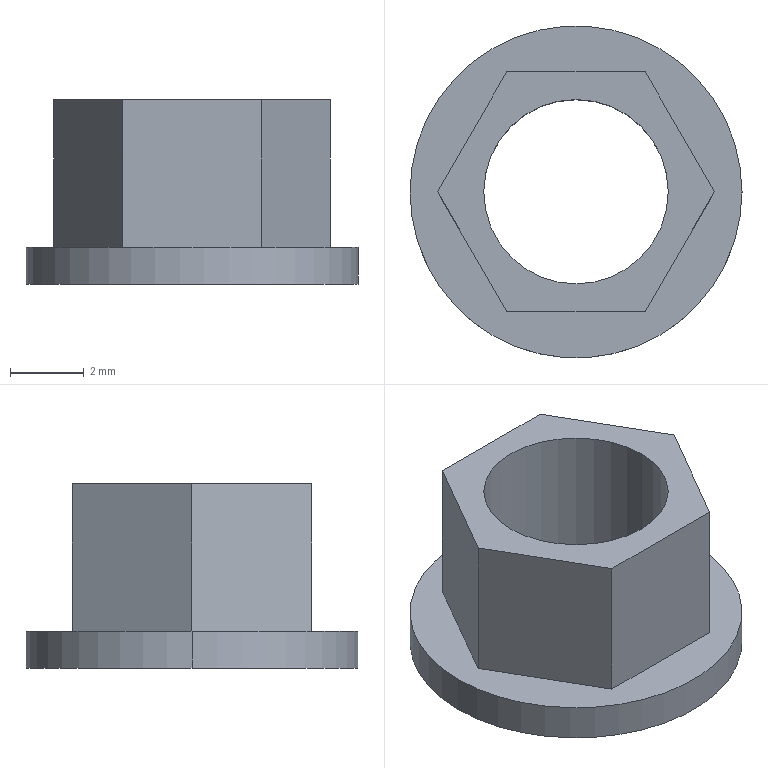Part | SolidWorks | features BaseBody 1 | 1 solid | 13 faces | box 9 x 9 x 5 mm | volume 111.801 mm3 | plane 9 | cylinder 4 | commonest cylinder face diameters 5 x2 9 x2
STEP:
#1=CARTESIAN_POINT('',(2.5,0.,0.));
#2=VERTEX_POINT('',#1);
#3=CARTESIAN_POINT('',(-2.5,0.,0.));
#4=VERTEX_POINT('',#3);
#5=CARTESIAN_POINT('',(0.,0.,0.));
#6=DIRECTION('',(0.,0.,1.));
#7=DIRECTION('',(-1.,0.,0.));
#8=AXIS2_PLACEMENT_3D('',#5,#6,#7);
#9=CIRCLE('',#8,2.5);
#10=EDGE_CURVE('',#2,#4,#9,.T.);
#11=ORIENTED_EDGE('',*,*,#10,.F.);
#12=CARTESIAN_POINT('',(2.5,0.,5.));
#13=VERTEX_POINT('',#12);
#14=CARTESIAN_POINT('',(2.5,0.,5.));
#15=DIRECTION('',(0.,0.,1.));
#16=VECTOR('',#15,1000.);
#17=LINE('',#14,#16);
#18=EDGE_CURVE('',#2,#13,#17,.T.);
#19=ORIENTED_EDGE('',*,*,#18,.T.);
#20=CARTESIAN_POINT('',(-2.5,0.,5.));
#21=VERTEX_POINT('',#20);
#22=CARTESIAN_POINT('',(0.,0.,5.));
#23=DIRECTION('',(0.,0.,-1.));
#24=DIRECTION('',(-1.,0.,0.));
#25=AXIS2_PLACEMENT_3D('',#22,#23,#24);
#26=CIRCLE('',#25,2.5);
#27=EDGE_CURVE('',#21,#13,#26,.T.);
#28=ORIENTED_EDGE('',*,*,#27,.F.);
#29=CARTESIAN_POINT('',(-2.5,0.,5.));
#30=DIRECTION('',(0.,0.,1.));
#31=VECTOR('',#30,1000.);
#32=LINE('',#29,#31);
#33=EDGE_CURVE('',#4,#21,#32,.T.);
#34=ORIENTED_EDGE('',*,*,#33,.F.);
#35=EDGE_LOOP('',(#11,#19,#28,#34));
#36=FACE_OUTER_BOUND('',#35,.T.);
#37=CARTESIAN_POINT('',(0.,0.,5.));
#38=DIRECTION('',(0.,0.,1.));
#39=DIRECTION('',(-1.,0.,0.));
#40=AXIS2_PLACEMENT_3D('',#37,#38,#39);
#41=CYLINDRICAL_SURFACE('',#40,2.5);
#42=ADVANCED_FACE('',(#36),#41,.F.);
#43=CARTESIAN_POINT('',(4.5,0.,1.));
#44=VERTEX_POINT('',#43);
#45=CARTESIAN_POINT('',(-4.5,0.,1.));
#46=VERTEX_POINT('',#45);
#47=CARTESIAN_POINT('',(0.,0.,1.));
#48=DIRECTION('',(0.,0.,1.));
#49=DIRECTION('',(-1.,0.,0.));
#50=AXIS2_PLACEMENT_3D('',#47,#48,#49);
#51=CIRCLE('',#50,4.5);
#52=EDGE_CURVE('',#44,#46,#51,.T.);
#53=ORIENTED_EDGE('',*,*,#52,.F.);
#54=CARTESIAN_POINT('',(4.5,0.,0.));
#55=VERTEX_POINT('',#54);
#56=CARTESIAN_POINT('',(4.5,0.,0.));
#57=DIRECTION('',(0.,0.,-1.));
#58=VECTOR('',#57,1000.);
#59=LINE('',#56,#58);
#60=EDGE_CURVE('',#44,#55,#59,.T.);
#61=ORIENTED_EDGE('',*,*,#60,.T.);
#62=CARTESIAN_POINT('',(-4.5,0.,0.));
#63=VERTEX_POINT('',#62);
#64=CARTESIAN_POINT('',(0.,0.,0.));
#65=DIRECTION('',(0.,0.,-1.));
#66=DIRECTION('',(-1.,0.,0.));
#67=AXIS2_PLACEMENT_3D('',#64,#65,#66);
#68=CIRCLE('',#67,4.5);
#69=EDGE_CURVE('',#63,#55,#68,.T.);
#70=ORIENTED_EDGE('',*,*,#69,.F.);
#71=CARTESIAN_POINT('',(-4.5,0.,0.));
#72=DIRECTION('',(0.,0.,-1.));
#73=VECTOR('',#72,1000.);
#74=LINE('',#71,#73);
#75=EDGE_CURVE('',#46,#63,#74,.T.);
#76=ORIENTED_EDGE('',*,*,#75,.F.);
#77=EDGE_LOOP('',(#53,#61,#70,#76));
#78=FACE_OUTER_BOUND('',#77,.T.);
#79=CARTESIAN_POINT('',(0.,0.,0.));
#80=DIRECTION('',(0.,0.,-1.));
#81=DIRECTION('',(-1.,0.,0.));
#82=AXIS2_PLACEMENT_3D('',#79,#80,#81);
#83=CYLINDRICAL_SURFACE('',#82,4.5);
#84=ADVANCED_FACE('',(#78),#83,.T.);
#85=CARTESIAN_POINT('',(-1.876,-3.25,1.));
#86=VERTEX_POINT('',#85);
#87=CARTESIAN_POINT('',(-3.753,0.,1.));
#88=VERTEX_POINT('',#87);
#89=CARTESIAN_POINT('',(-3.284,-0.8125,1.));
#90=DIRECTION('',(-0.5,0.866,0.));
#91=VECTOR('',#90,1000.);
#92=LINE('',#89,#91);
#93=EDGE_CURVE('',#86,#88,#92,.T.);
#94=ORIENTED_EDGE('',*,*,#93,.F.);
#95=CARTESIAN_POINT('',(-1.876,-3.25,5.));
#96=VERTEX_POINT('',#95);
#97=CARTESIAN_POINT('',(-1.876,-3.25,1.));
#98=DIRECTION('',(0.,0.,1.));
#99=VECTOR('',#98,1000.);
#100=LINE('',#97,#99);
#101=EDGE_CURVE('',#86,#96,#100,.T.);
#102=ORIENTED_EDGE('',*,*,#101,.T.);
#103=CARTESIAN_POINT('',(-3.753,0.,5.));
#104=VERTEX_POINT('',#103);
#105=CARTESIAN_POINT('',(-1.876,-3.25,5.));
#106=DIRECTION('',(0.5,-0.866,0.));
#107=VECTOR('',#106,1000.);
#108=LINE('',#105,#107);
#109=EDGE_CURVE('',#104,#96,#108,.T.);
#110=ORIENTED_EDGE('',*,*,#109,.F.);
#111=CARTESIAN_POINT('',(-3.753,0.,1.));
#112=DIRECTION('',(0.,0.,1.));
#113=VECTOR('',#112,1000.);
#114=LINE('',#111,#113);
#115=EDGE_CURVE('',#88,#104,#114,.T.);
#116=ORIENTED_EDGE('',*,*,#115,.F.);
#117=EDGE_LOOP('',(#94,#102,#110,#116));
#118=FACE_OUTER_BOUND('',#117,.T.);
#119=CARTESIAN_POINT('',(-3.753,0.,1.));
#120=DIRECTION('',(-0.866,-0.5,0.));
#121=DIRECTION('',(-0.5,0.866,0.));
#122=AXIS2_PLACEMENT_3D('',#119,#120,#121);
#123=PLANE('',#122);
#124=ADVANCED_FACE('',(#118),#123,.T.);
#125=CARTESIAN_POINT('',(-1.876,3.25,1.));
#126=VERTEX_POINT('',#125);
#127=CARTESIAN_POINT('',(-2.345,2.438,1.));
#128=DIRECTION('',(0.5,0.866,0.));
#129=VECTOR('',#128,1000.);
#130=LINE('',#127,#129);
#131=EDGE_CURVE('',#88,#126,#130,.T.);
#132=ORIENTED_EDGE('',*,*,#131,.F.);
#133=ORIENTED_EDGE('',*,*,#115,.T.);
#134=CARTESIAN_POINT('',(-1.876,3.25,5.));
#135=VERTEX_POINT('',#134);
#136=CARTESIAN_POINT('',(-3.753,0.,5.));
#137=DIRECTION('',(-0.5,-0.866,0.));
#138=VECTOR('',#137,1000.);
#139=LINE('',#136,#138);
#140=EDGE_CURVE('',#135,#104,#139,.T.);
#141=ORIENTED_EDGE('',*,*,#140,.F.);
#142=CARTESIAN_POINT('',(-1.876,3.25,1.));
#143=DIRECTION('',(0.,0.,1.));
#144=VECTOR('',#143,1000.);
#145=LINE('',#142,#144);
#146=EDGE_CURVE('',#126,#135,#145,.T.);
#147=ORIENTED_EDGE('',*,*,#146,.F.);
#148=EDGE_LOOP('',(#132,#133,#141,#147));
#149=FACE_OUTER_BOUND('',#148,.T.);
#150=CARTESIAN_POINT('',(-1.876,3.25,1.));
#151=DIRECTION('',(-0.866,0.5,0.));
#152=DIRECTION('',(0.,0.,1.));
#153=AXIS2_PLACEMENT_3D('',#150,#151,#152);
#154=PLANE('',#153);
#155=ADVANCED_FACE('',(#149),#154,.T.);
#156=CARTESIAN_POINT('',(1.876,3.25,1.));
#157=VERTEX_POINT('',#156);
#158=CARTESIAN_POINT('',(0.9382,3.25,1.));
#159=DIRECTION('',(1.,0.,0.));
#160=VECTOR('',#159,1000.);
#161=LINE('',#158,#160);
#162=EDGE_CURVE('',#126,#157,#161,.T.);
#163=ORIENTED_EDGE('',*,*,#162,.F.);
#164=ORIENTED_EDGE('',*,*,#146,.T.);
#165=CARTESIAN_POINT('',(1.876,3.25,5.));
#166=VERTEX_POINT('',#165);
#167=CARTESIAN_POINT('',(-1.876,3.25,5.));
#168=DIRECTION('',(-1.,0.,0.));
#169=VECTOR('',#168,1000.);
#170=LINE('',#167,#169);
#171=EDGE_CURVE('',#166,#135,#170,.T.);
#172=ORIENTED_EDGE('',*,*,#171,.F.);
#173=CARTESIAN_POINT('',(1.876,3.25,1.));
#174=DIRECTION('',(0.,0.,1.));
#175=VECTOR('',#174,1000.);
#176=LINE('',#173,#175);
#177=EDGE_CURVE('',#157,#166,#176,.T.);
#178=ORIENTED_EDGE('',*,*,#177,.F.);
#179=EDGE_LOOP('',(#163,#164,#172,#178));
#180=FACE_OUTER_BOUND('',#179,.T.);
#181=CARTESIAN_POINT('',(1.876,3.25,1.));
#182=DIRECTION('',(0.,1.,0.));
#183=DIRECTION('',(1.,0.,0.));
#184=AXIS2_PLACEMENT_3D('',#181,#182,#183);
#185=PLANE('',#184);
#186=ADVANCED_FACE('',(#180),#185,.T.);
#187=CARTESIAN_POINT('',(3.753,0.,1.));
#188=VERTEX_POINT('',#187);
#189=CARTESIAN_POINT('',(3.284,0.8125,1.));
#190=DIRECTION('',(0.5,-0.866,0.));
#191=VECTOR('',#190,1000.);
#192=LINE('',#189,#191);
#193=EDGE_CURVE('',#157,#188,#192,.T.);
#194=ORIENTED_EDGE('',*,*,#193,.F.);
#195=ORIENTED_EDGE('',*,*,#177,.T.);
#196=CARTESIAN_POINT('',(3.753,0.,5.));
#197=VERTEX_POINT('',#196);
#198=CARTESIAN_POINT('',(1.876,3.25,5.));
#199=DIRECTION('',(-0.5,0.866,0.));
#200=VECTOR('',#199,1000.);
#201=LINE('',#198,#200);
#202=EDGE_CURVE('',#197,#166,#201,.T.);
#203=ORIENTED_EDGE('',*,*,#202,.F.);
#204=CARTESIAN_POINT('',(3.753,0.,1.));
#205=DIRECTION('',(0.,0.,1.));
#206=VECTOR('',#205,1000.);
#207=LINE('',#204,#206);
#208=EDGE_CURVE('',#188,#197,#207,.T.);
#209=ORIENTED_EDGE('',*,*,#208,.F.);
#210=EDGE_LOOP('',(#194,#195,#203,#209));
#211=FACE_OUTER_BOUND('',#210,.T.);
#212=CARTESIAN_POINT('',(3.753,0.,1.));
#213=DIRECTION('',(0.866,0.5,0.));
#214=DIRECTION('',(0.,0.,-1.));
#215=AXIS2_PLACEMENT_3D('',#212,#213,#214);
#216=PLANE('',#215);
#217=ADVANCED_FACE('',(#211),#216,.T.);
#218=CARTESIAN_POINT('',(1.876,-3.25,1.));
#219=VERTEX_POINT('',#218);
#220=CARTESIAN_POINT('',(2.345,-2.438,1.));
#221=DIRECTION('',(-0.5,-0.866,0.));
#222=VECTOR('',#221,1000.);
#223=LINE('',#220,#222);
#224=EDGE_CURVE('',#188,#219,#223,.T.);
#225=ORIENTED_EDGE('',*,*,#224,.F.);
#226=ORIENTED_EDGE('',*,*,#208,.T.);
#227=CARTESIAN_POINT('',(1.876,-3.25,5.));
#228=VERTEX_POINT('',#227);
#229=CARTESIAN_POINT('',(3.753,0.,5.));
#230=DIRECTION('',(0.5,0.866,0.));
#231=VECTOR('',#230,1000.);
#232=LINE('',#229,#231);
#233=EDGE_CURVE('',#228,#197,#232,.T.);
#234=ORIENTED_EDGE('',*,*,#233,.F.);
#235=CARTESIAN_POINT('',(1.876,-3.25,1.));
#236=DIRECTION('',(0.,0.,1.));
#237=VECTOR('',#236,1000.);
#238=LINE('',#235,#237);
#239=EDGE_CURVE('',#219,#228,#238,.T.);
#240=ORIENTED_EDGE('',*,*,#239,.F.);
#241=EDGE_LOOP('',(#225,#226,#234,#240));
#242=FACE_OUTER_BOUND('',#241,.T.);
#243=CARTESIAN_POINT('',(1.876,-3.25,1.));
#244=DIRECTION('',(0.866,-0.5,0.));
#245=DIRECTION('',(0.,0.,-1.));
#246=AXIS2_PLACEMENT_3D('',#243,#244,#245);
#247=PLANE('',#246);
#248=ADVANCED_FACE('',(#242),#247,.T.);
#249=CARTESIAN_POINT('',(-0.9382,-3.25,1.));
#250=DIRECTION('',(-1.,0.,0.));
#251=VECTOR('',#250,1000.);
#252=LINE('',#249,#251);
#253=EDGE_CURVE('',#219,#86,#252,.T.);
#254=ORIENTED_EDGE('',*,*,#253,.F.);
#255=ORIENTED_EDGE('',*,*,#239,.T.);
#256=CARTESIAN_POINT('',(1.876,-3.25,5.));
#257=DIRECTION('',(1.,0.,0.));
#258=VECTOR('',#257,1000.);
#259=LINE('',#256,#258);
#260=EDGE_CURVE('',#96,#228,#259,.T.);
#261=ORIENTED_EDGE('',*,*,#260,.F.);
#262=ORIENTED_EDGE('',*,*,#101,.F.);
#263=EDGE_LOOP('',(#254,#255,#261,#262));
#264=FACE_OUTER_BOUND('',#263,.T.);
#265=CARTESIAN_POINT('',(-1.876,-3.25,1.));
#266=DIRECTION('',(0.,-1.,0.));
#267=DIRECTION('',(-1.,0.,0.));
#268=AXIS2_PLACEMENT_3D('',#265,#266,#267);
#269=PLANE('',#268);
#270=ADVANCED_FACE('',(#264),#269,.T.);
#271=ORIENTED_EDGE('',*,*,#27,.T.);
#272=CARTESIAN_POINT('',(0.,0.,5.));
#273=DIRECTION('',(0.,0.,-1.));
#274=DIRECTION('',(-1.,0.,0.));
#275=AXIS2_PLACEMENT_3D('',#272,#273,#274);
#276=CIRCLE('',#275,2.5);
#277=EDGE_CURVE('',#13,#21,#276,.T.);
#278=ORIENTED_EDGE('',*,*,#277,.T.);
#279=EDGE_LOOP('',(#271,#278));
#280=FACE_BOUND('',#279,.T.);
#281=ORIENTED_EDGE('',*,*,#260,.T.);
#282=ORIENTED_EDGE('',*,*,#233,.T.);
#283=ORIENTED_EDGE('',*,*,#202,.T.);
#284=ORIENTED_EDGE('',*,*,#171,.T.);
#285=ORIENTED_EDGE('',*,*,#140,.T.);
#286=ORIENTED_EDGE('',*,*,#109,.T.);
#287=EDGE_LOOP('',(#281,#282,#283,#284,#285,#286));
#288=FACE_OUTER_BOUND('',#287,.T.);
#289=CARTESIAN_POINT('',(0.,0.,5.));
#290=DIRECTION('',(0.,0.,1.));
#291=DIRECTION('',(1.,0.,0.));
#292=AXIS2_PLACEMENT_3D('',#289,#290,#291);
#293=PLANE('',#292);
#294=ADVANCED_FACE('',(#280,#288),#293,.T.);
#295=CARTESIAN_POINT('',(0.,0.,0.));
#296=DIRECTION('',(0.,0.,1.));
#297=DIRECTION('',(-1.,0.,0.));
#298=AXIS2_PLACEMENT_3D('',#295,#296,#297);
#299=CIRCLE('',#298,2.5);
#300=EDGE_CURVE('',#4,#2,#299,.T.);
#301=ORIENTED_EDGE('',*,*,#300,.T.);
#302=ORIENTED_EDGE('',*,*,#10,.T.);
#303=EDGE_LOOP('',(#301,#302));
#304=FACE_BOUND('',#303,.T.);
#305=ORIENTED_EDGE('',*,*,#69,.T.);
#306=CARTESIAN_POINT('',(0.,0.,0.));
#307=DIRECTION('',(0.,0.,-1.));
#308=DIRECTION('',(-1.,0.,0.));
#309=AXIS2_PLACEMENT_3D('',#306,#307,#308);
#310=CIRCLE('',#309,4.5);
#311=EDGE_CURVE('',#55,#63,#310,.T.);
#312=ORIENTED_EDGE('',*,*,#311,.T.);
#313=EDGE_LOOP('',(#305,#312));
#314=FACE_OUTER_BOUND('',#313,.T.);
#315=CARTESIAN_POINT('',(0.,0.,0.));
#316=DIRECTION('',(0.,0.,1.));
#317=DIRECTION('',(1.,0.,0.));
#318=AXIS2_PLACEMENT_3D('',#315,#316,#317);
#319=PLANE('',#318);
#320=ADVANCED_FACE('',(#304,#314),#319,.F.);
#321=ORIENTED_EDGE('',*,*,#93,.T.);
#322=ORIENTED_EDGE('',*,*,#131,.T.);
#323=ORIENTED_EDGE('',*,*,#162,.T.);
#324=ORIENTED_EDGE('',*,*,#193,.T.);
#325=ORIENTED_EDGE('',*,*,#224,.T.);
#326=ORIENTED_EDGE('',*,*,#253,.T.);
#327=EDGE_LOOP('',(#321,#322,#323,#324,#325,#326));
#328=FACE_BOUND('',#327,.T.);
#329=CARTESIAN_POINT('',(0.,0.,1.));
#330=DIRECTION('',(0.,0.,1.));
#331=DIRECTION('',(-1.,0.,0.));
#332=AXIS2_PLACEMENT_3D('',#329,#330,#331);
#333=CIRCLE('',#332,4.5);
#334=EDGE_CURVE('',#46,#44,#333,.T.);
#335=ORIENTED_EDGE('',*,*,#334,.T.);
#336=ORIENTED_EDGE('',*,*,#52,.T.);
#337=EDGE_LOOP('',(#335,#336));
#338=FACE_OUTER_BOUND('',#337,.T.);
#339=CARTESIAN_POINT('',(0.,0.,1.));
#340=DIRECTION('',(0.,0.,1.));
#341=DIRECTION('',(1.,0.,0.));
#342=AXIS2_PLACEMENT_3D('',#339,#340,#341);
#343=PLANE('',#342);
#344=ADVANCED_FACE('',(#328,#338),#343,.T.);
#345=ORIENTED_EDGE('',*,*,#60,.F.);
#346=ORIENTED_EDGE('',*,*,#334,.F.);
#347=ORIENTED_EDGE('',*,*,#75,.T.);
#348=ORIENTED_EDGE('',*,*,#311,.F.);
#349=EDGE_LOOP('',(#345,#346,#347,#348));
#350=FACE_OUTER_BOUND('',#349,.T.);
#351=CARTESIAN_POINT('',(0.,0.,0.));
#352=DIRECTION('',(0.,0.,-1.));
#353=DIRECTION('',(-1.,0.,0.));
#354=AXIS2_PLACEMENT_3D('',#351,#352,#353);
#355=CYLINDRICAL_SURFACE('',#354,4.5);
#356=ADVANCED_FACE('',(#350),#355,.T.);
#357=ORIENTED_EDGE('',*,*,#18,.F.);
#358=ORIENTED_EDGE('',*,*,#300,.F.);
#359=ORIENTED_EDGE('',*,*,#33,.T.);
#360=ORIENTED_EDGE('',*,*,#277,.F.);
#361=EDGE_LOOP('',(#357,#358,#359,#360));
#362=FACE_OUTER_BOUND('',#361,.T.);
#363=CARTESIAN_POINT('',(0.,0.,5.));
#364=DIRECTION('',(0.,0.,1.));
#365=DIRECTION('',(-1.,0.,0.));
#366=AXIS2_PLACEMENT_3D('',#363,#364,#365);
#367=CYLINDRICAL_SURFACE('',#366,2.5);
#368=ADVANCED_FACE('',(#362),#367,.F.);
#369=CLOSED_SHELL('',(#42,#84,#124,#155,#186,#217,#248,#270,#294,#320,#344,#356,#368));
#370=MANIFOLD_SOLID_BREP('',#369);
#371=CARTESIAN_POINT('',(0.,0.,0.));
#372=DIRECTION('',(0.,0.,1.));
#373=DIRECTION('',(1.,0.,0.));
#374=AXIS2_PLACEMENT_3D('',#371,#372,#373);
#375=(LENGTH_UNIT()NAMED_UNIT(*)SI_UNIT(.MILLI.,.METRE.));
#376=UNCERTAINTY_MEASURE_WITH_UNIT(LENGTH_MEASURE(0.00001),#375,'','');
#377=(NAMED_UNIT(*)PLANE_ANGLE_UNIT()SI_UNIT($,.RADIAN.));
#378=(NAMED_UNIT(*)SI_UNIT($,.STERADIAN.)SOLID_ANGLE_UNIT());
#379=(GEOMETRIC_REPRESENTATION_CONTEXT(3)GLOBAL_UNCERTAINTY_ASSIGNED_CONTEXT((#376))GLOBAL_UNIT_ASSIGNED_CONTEXT((#375,#377,#378))REPRESENTATION_CONTEXT('',''));
#380=ADVANCED_BREP_SHAPE_REPRESENTATION('',(#370,#374),#379);